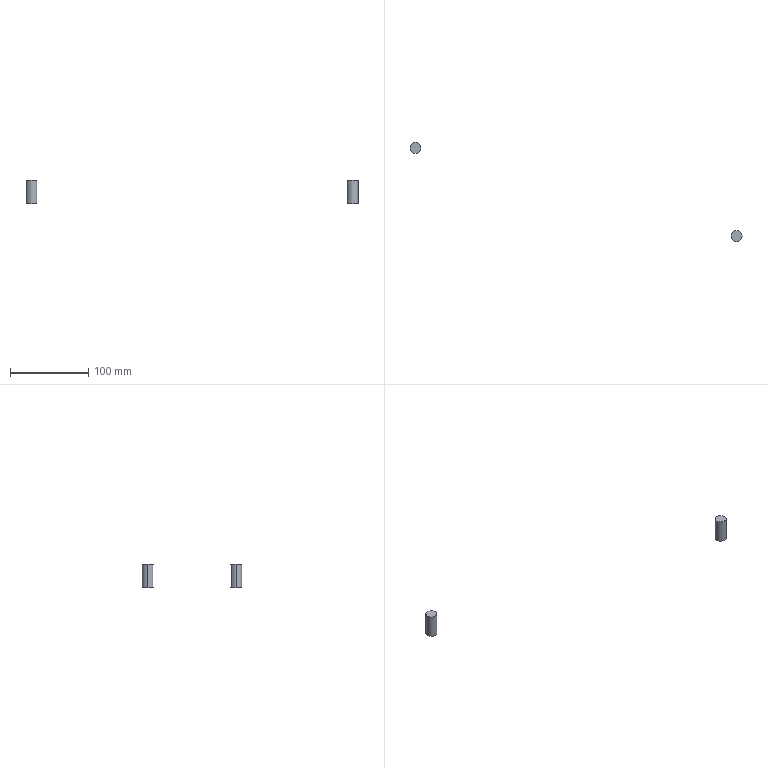Part | SolidWorks | features Extrusion 1 | 2 solids | 8 faces | box 423.435 x 126.4 x 30 mm | volume 9236 mm3 | cylinder 4 | plane 4 | commonest cylinder face diameters 14 x4
STEP:
#1=CARTESIAN_POINT('',(636.,379.878,30.));
#2=VERTEX_POINT('',#1);
#3=CARTESIAN_POINT('',(622.,379.878,30.));
#4=VERTEX_POINT('',#3);
#5=CARTESIAN_POINT('',(629.,379.878,30.));
#6=DIRECTION('',(0.,0.,1.));
#7=DIRECTION('',(1.,0.,0.));
#8=AXIS2_PLACEMENT_3D('',#5,#6,#7);
#9=CIRCLE('',#8,7.);
#10=EDGE_CURVE('',#2,#4,#9,.T.);
#11=ORIENTED_EDGE('',*,*,#10,.F.);
#12=CARTESIAN_POINT('',(636.,379.878,0.));
#13=VERTEX_POINT('',#12);
#14=CARTESIAN_POINT('',(636.,379.878,30.));
#15=DIRECTION('',(0.,0.,-1.));
#16=VECTOR('',#15,1000.);
#17=LINE('',#14,#16);
#18=EDGE_CURVE('',#2,#13,#17,.T.);
#19=ORIENTED_EDGE('',*,*,#18,.T.);
#20=CARTESIAN_POINT('',(622.,379.878,0.));
#21=VERTEX_POINT('',#20);
#22=CARTESIAN_POINT('',(629.,379.878,0.));
#23=DIRECTION('',(0.,0.,1.));
#24=DIRECTION('',(1.,0.,0.));
#25=AXIS2_PLACEMENT_3D('',#22,#23,#24);
#26=CIRCLE('',#25,7.);
#27=EDGE_CURVE('',#13,#21,#26,.T.);
#28=ORIENTED_EDGE('',*,*,#27,.T.);
#29=CARTESIAN_POINT('',(622.,379.878,30.));
#30=DIRECTION('',(0.,0.,-1.));
#31=VECTOR('',#30,1000.);
#32=LINE('',#29,#31);
#33=EDGE_CURVE('',#4,#21,#32,.T.);
#34=ORIENTED_EDGE('',*,*,#33,.F.);
#35=EDGE_LOOP('',(#11,#19,#28,#34));
#36=FACE_OUTER_BOUND('',#35,.T.);
#37=CARTESIAN_POINT('',(629.,379.878,30.));
#38=DIRECTION('',(0.,0.,-1.));
#39=DIRECTION('',(-1.,0.,0.));
#40=AXIS2_PLACEMENT_3D('',#37,#38,#39);
#41=CYLINDRICAL_SURFACE('',#40,7.);
#42=ADVANCED_FACE('',(#36),#41,.T.);
#43=ORIENTED_EDGE('',*,*,#18,.F.);
#44=CARTESIAN_POINT('',(629.,379.878,30.));
#45=DIRECTION('',(0.,0.,1.));
#46=DIRECTION('',(1.,0.,0.));
#47=AXIS2_PLACEMENT_3D('',#44,#45,#46);
#48=CIRCLE('',#47,7.);
#49=EDGE_CURVE('',#4,#2,#48,.T.);
#50=ORIENTED_EDGE('',*,*,#49,.F.);
#51=ORIENTED_EDGE('',*,*,#33,.T.);
#52=CARTESIAN_POINT('',(629.,379.878,0.));
#53=DIRECTION('',(0.,0.,1.));
#54=DIRECTION('',(1.,0.,0.));
#55=AXIS2_PLACEMENT_3D('',#52,#53,#54);
#56=CIRCLE('',#55,7.);
#57=EDGE_CURVE('',#21,#13,#56,.T.);
#58=ORIENTED_EDGE('',*,*,#57,.T.);
#59=EDGE_LOOP('',(#43,#50,#51,#58));
#60=FACE_OUTER_BOUND('',#59,.T.);
#61=CARTESIAN_POINT('',(629.,379.878,30.));
#62=DIRECTION('',(0.,0.,-1.));
#63=DIRECTION('',(-1.,0.,0.));
#64=AXIS2_PLACEMENT_3D('',#61,#62,#63);
#65=CYLINDRICAL_SURFACE('',#64,7.);
#66=ADVANCED_FACE('',(#60),#65,.T.);
#67=ORIENTED_EDGE('',*,*,#49,.T.);
#68=ORIENTED_EDGE('',*,*,#10,.T.);
#69=EDGE_LOOP('',(#67,#68));
#70=FACE_OUTER_BOUND('',#69,.T.);
#71=CARTESIAN_POINT('',(629.,379.878,30.));
#72=DIRECTION('',(0.,0.,1.));
#73=DIRECTION('',(1.,0.,0.));
#74=AXIS2_PLACEMENT_3D('',#71,#72,#73);
#75=PLANE('',#74);
#76=ADVANCED_FACE('',(#70),#75,.T.);
#77=ORIENTED_EDGE('',*,*,#57,.F.);
#78=ORIENTED_EDGE('',*,*,#27,.F.);
#79=EDGE_LOOP('',(#77,#78));
#80=FACE_OUTER_BOUND('',#79,.T.);
#81=CARTESIAN_POINT('',(629.,379.878,0.));
#82=DIRECTION('',(0.,0.,1.));
#83=DIRECTION('',(1.,0.,0.));
#84=AXIS2_PLACEMENT_3D('',#81,#82,#83);
#85=PLANE('',#84);
#86=ADVANCED_FACE('',(#80),#85,.F.);
#87=CLOSED_SHELL('',(#42,#66,#76,#86));
#88=MANIFOLD_SOLID_BREP('',#87);
#89=CARTESIAN_POINT('',(226.565,492.278,30.));
#90=VERTEX_POINT('',#89);
#91=CARTESIAN_POINT('',(212.565,492.278,30.));
#92=VERTEX_POINT('',#91);
#93=CARTESIAN_POINT('',(219.565,492.278,30.));
#94=DIRECTION('',(0.,0.,1.));
#95=DIRECTION('',(1.,0.,0.));
#96=AXIS2_PLACEMENT_3D('',#93,#94,#95);
#97=CIRCLE('',#96,7.);
#98=EDGE_CURVE('',#90,#92,#97,.T.);
#99=ORIENTED_EDGE('',*,*,#98,.F.);
#100=CARTESIAN_POINT('',(226.565,492.278,0.));
#101=VERTEX_POINT('',#100);
#102=CARTESIAN_POINT('',(226.565,492.278,30.));
#103=DIRECTION('',(0.,0.,-1.));
#104=VECTOR('',#103,1000.);
#105=LINE('',#102,#104);
#106=EDGE_CURVE('',#90,#101,#105,.T.);
#107=ORIENTED_EDGE('',*,*,#106,.T.);
#108=CARTESIAN_POINT('',(212.565,492.278,0.));
#109=VERTEX_POINT('',#108);
#110=CARTESIAN_POINT('',(219.565,492.278,0.));
#111=DIRECTION('',(0.,0.,1.));
#112=DIRECTION('',(1.,0.,0.));
#113=AXIS2_PLACEMENT_3D('',#110,#111,#112);
#114=CIRCLE('',#113,7.);
#115=EDGE_CURVE('',#101,#109,#114,.T.);
#116=ORIENTED_EDGE('',*,*,#115,.T.);
#117=CARTESIAN_POINT('',(212.565,492.278,30.));
#118=DIRECTION('',(0.,0.,-1.));
#119=VECTOR('',#118,1000.);
#120=LINE('',#117,#119);
#121=EDGE_CURVE('',#92,#109,#120,.T.);
#122=ORIENTED_EDGE('',*,*,#121,.F.);
#123=EDGE_LOOP('',(#99,#107,#116,#122));
#124=FACE_OUTER_BOUND('',#123,.T.);
#125=CARTESIAN_POINT('',(219.565,492.278,30.));
#126=DIRECTION('',(0.,0.,-1.));
#127=DIRECTION('',(-1.,0.,0.));
#128=AXIS2_PLACEMENT_3D('',#125,#126,#127);
#129=CYLINDRICAL_SURFACE('',#128,7.);
#130=ADVANCED_FACE('',(#124),#129,.T.);
#131=ORIENTED_EDGE('',*,*,#106,.F.);
#132=CARTESIAN_POINT('',(219.565,492.278,30.));
#133=DIRECTION('',(0.,0.,1.));
#134=DIRECTION('',(1.,0.,0.));
#135=AXIS2_PLACEMENT_3D('',#132,#133,#134);
#136=CIRCLE('',#135,7.);
#137=EDGE_CURVE('',#92,#90,#136,.T.);
#138=ORIENTED_EDGE('',*,*,#137,.F.);
#139=ORIENTED_EDGE('',*,*,#121,.T.);
#140=CARTESIAN_POINT('',(219.565,492.278,0.));
#141=DIRECTION('',(0.,0.,1.));
#142=DIRECTION('',(1.,0.,0.));
#143=AXIS2_PLACEMENT_3D('',#140,#141,#142);
#144=CIRCLE('',#143,7.);
#145=EDGE_CURVE('',#109,#101,#144,.T.);
#146=ORIENTED_EDGE('',*,*,#145,.T.);
#147=EDGE_LOOP('',(#131,#138,#139,#146));
#148=FACE_OUTER_BOUND('',#147,.T.);
#149=CARTESIAN_POINT('',(219.565,492.278,30.));
#150=DIRECTION('',(0.,0.,-1.));
#151=DIRECTION('',(-1.,0.,0.));
#152=AXIS2_PLACEMENT_3D('',#149,#150,#151);
#153=CYLINDRICAL_SURFACE('',#152,7.);
#154=ADVANCED_FACE('',(#148),#153,.T.);
#155=ORIENTED_EDGE('',*,*,#137,.T.);
#156=ORIENTED_EDGE('',*,*,#98,.T.);
#157=EDGE_LOOP('',(#155,#156));
#158=FACE_OUTER_BOUND('',#157,.T.);
#159=CARTESIAN_POINT('',(219.565,492.278,30.));
#160=DIRECTION('',(0.,0.,1.));
#161=DIRECTION('',(1.,0.,0.));
#162=AXIS2_PLACEMENT_3D('',#159,#160,#161);
#163=PLANE('',#162);
#164=ADVANCED_FACE('',(#158),#163,.T.);
#165=ORIENTED_EDGE('',*,*,#145,.F.);
#166=ORIENTED_EDGE('',*,*,#115,.F.);
#167=EDGE_LOOP('',(#165,#166));
#168=FACE_OUTER_BOUND('',#167,.T.);
#169=CARTESIAN_POINT('',(219.565,492.278,0.));
#170=DIRECTION('',(0.,0.,1.));
#171=DIRECTION('',(1.,0.,0.));
#172=AXIS2_PLACEMENT_3D('',#169,#170,#171);
#173=PLANE('',#172);
#174=ADVANCED_FACE('',(#168),#173,.F.);
#175=CLOSED_SHELL('',(#130,#154,#164,#174));
#176=MANIFOLD_SOLID_BREP('',#175);
#177=CARTESIAN_POINT('',(0.,0.,0.));
#178=DIRECTION('',(0.,0.,1.));
#179=DIRECTION('',(1.,0.,0.));
#180=AXIS2_PLACEMENT_3D('',#177,#178,#179);
#181=(LENGTH_UNIT()NAMED_UNIT(*)SI_UNIT(.MILLI.,.METRE.));
#182=UNCERTAINTY_MEASURE_WITH_UNIT(LENGTH_MEASURE(0.00001),#181,'','');
#183=(NAMED_UNIT(*)PLANE_ANGLE_UNIT()SI_UNIT($,.RADIAN.));
#184=(NAMED_UNIT(*)SI_UNIT($,.STERADIAN.)SOLID_ANGLE_UNIT());
#185=(GEOMETRIC_REPRESENTATION_CONTEXT(3)GLOBAL_UNCERTAINTY_ASSIGNED_CONTEXT((#182))GLOBAL_UNIT_ASSIGNED_CONTEXT((#181,#183,#184))REPRESENTATION_CONTEXT('',''));
#186=ADVANCED_BREP_SHAPE_REPRESENTATION('',(#88,#176,#180),#185);